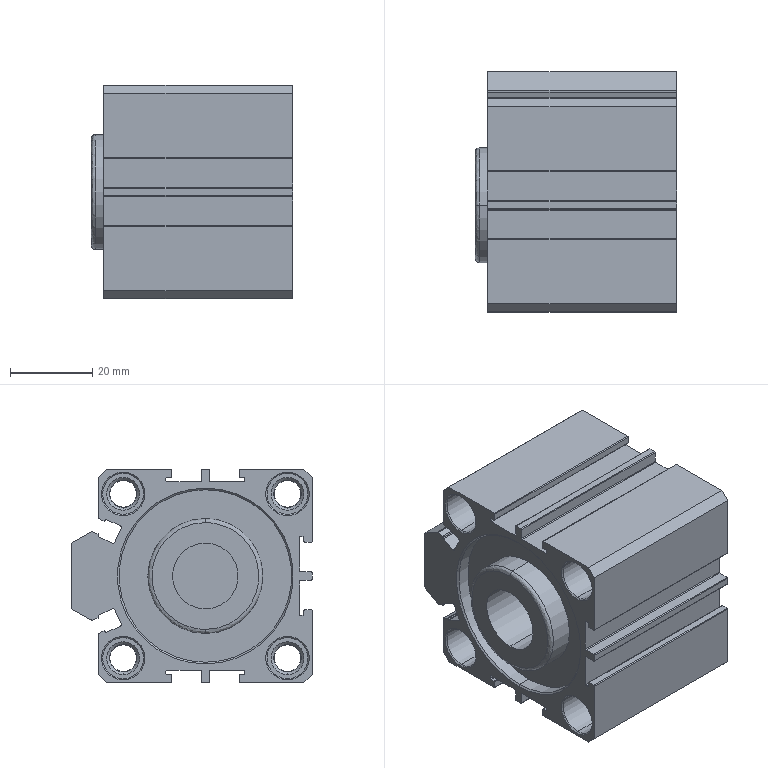Part | SolidWorks | features BaseBody 1 | 1 solid | 255 faces | box 49 x 58.5 x 52 mm | volume 67362 mm3 | cylinder 110 | plane 87 | cone 56 | spline 2 | commonest cylinder face diameters 0.4 x46 6.647 x16 10 x16 0.8 x10 6.5 x8 8.566 x4